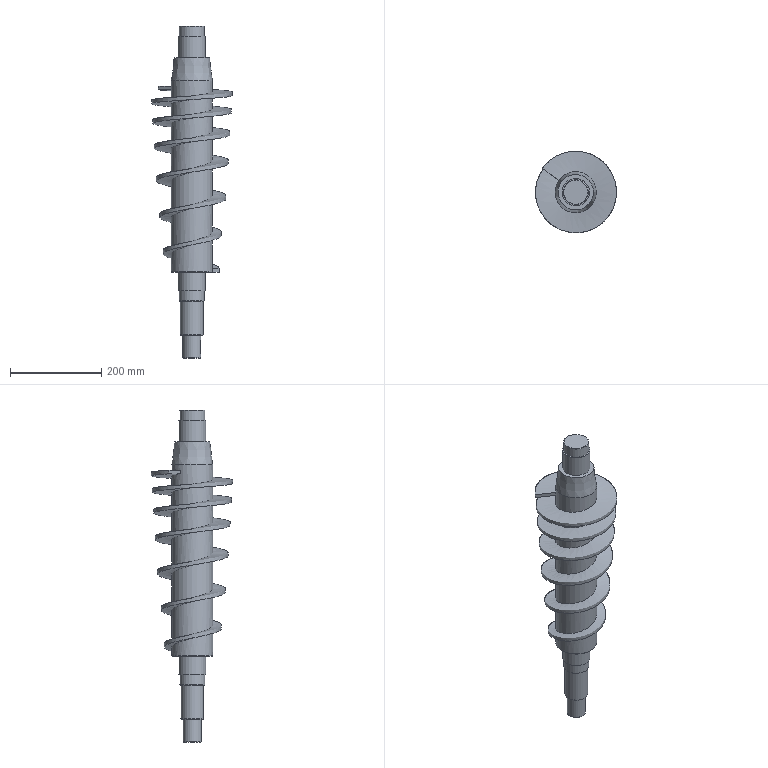Part | NX | features CYLINDER 7, DATUM_CSYS 4, CHAMFER 2, SKETCH 2, UNITE 2, EXTRUDE 1, HELIX 1, LINE 1, SKIN 1 | 1 solid | 36 faces | box 177.285 x 178.372 x 728 mm | volume 4210187 mm3 | cylinder 15 | plane 13 | cone 6 | spline 2 | commonest cylinder face diameters 90 x7 12 x2 55 x2 60 x2 40 x1 50 x1